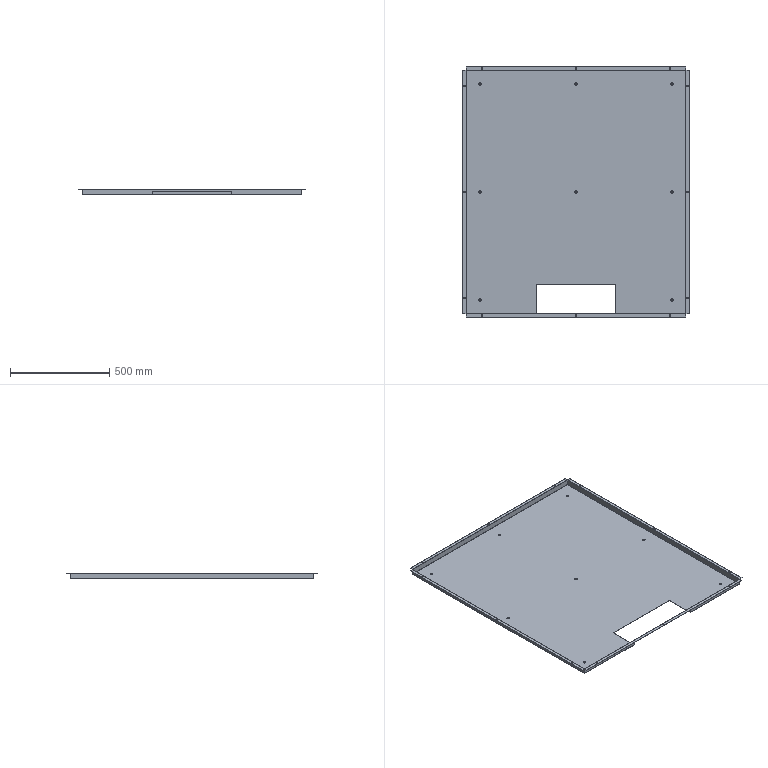Part | SolidWorks | features ICE 3, EdgeFlange 2, FlatPattern 1, SMBaseFlange 1, SheetMetal 1 | 1 solid | 150 faces | box 1140 x 1260 x 30 mm | volume 1498692 mm3 | plane 78 | cylinder 64 | spline 8 | commonest cylinder face diameters 7 x30 11 x16 0.4 x9 2.4 x9